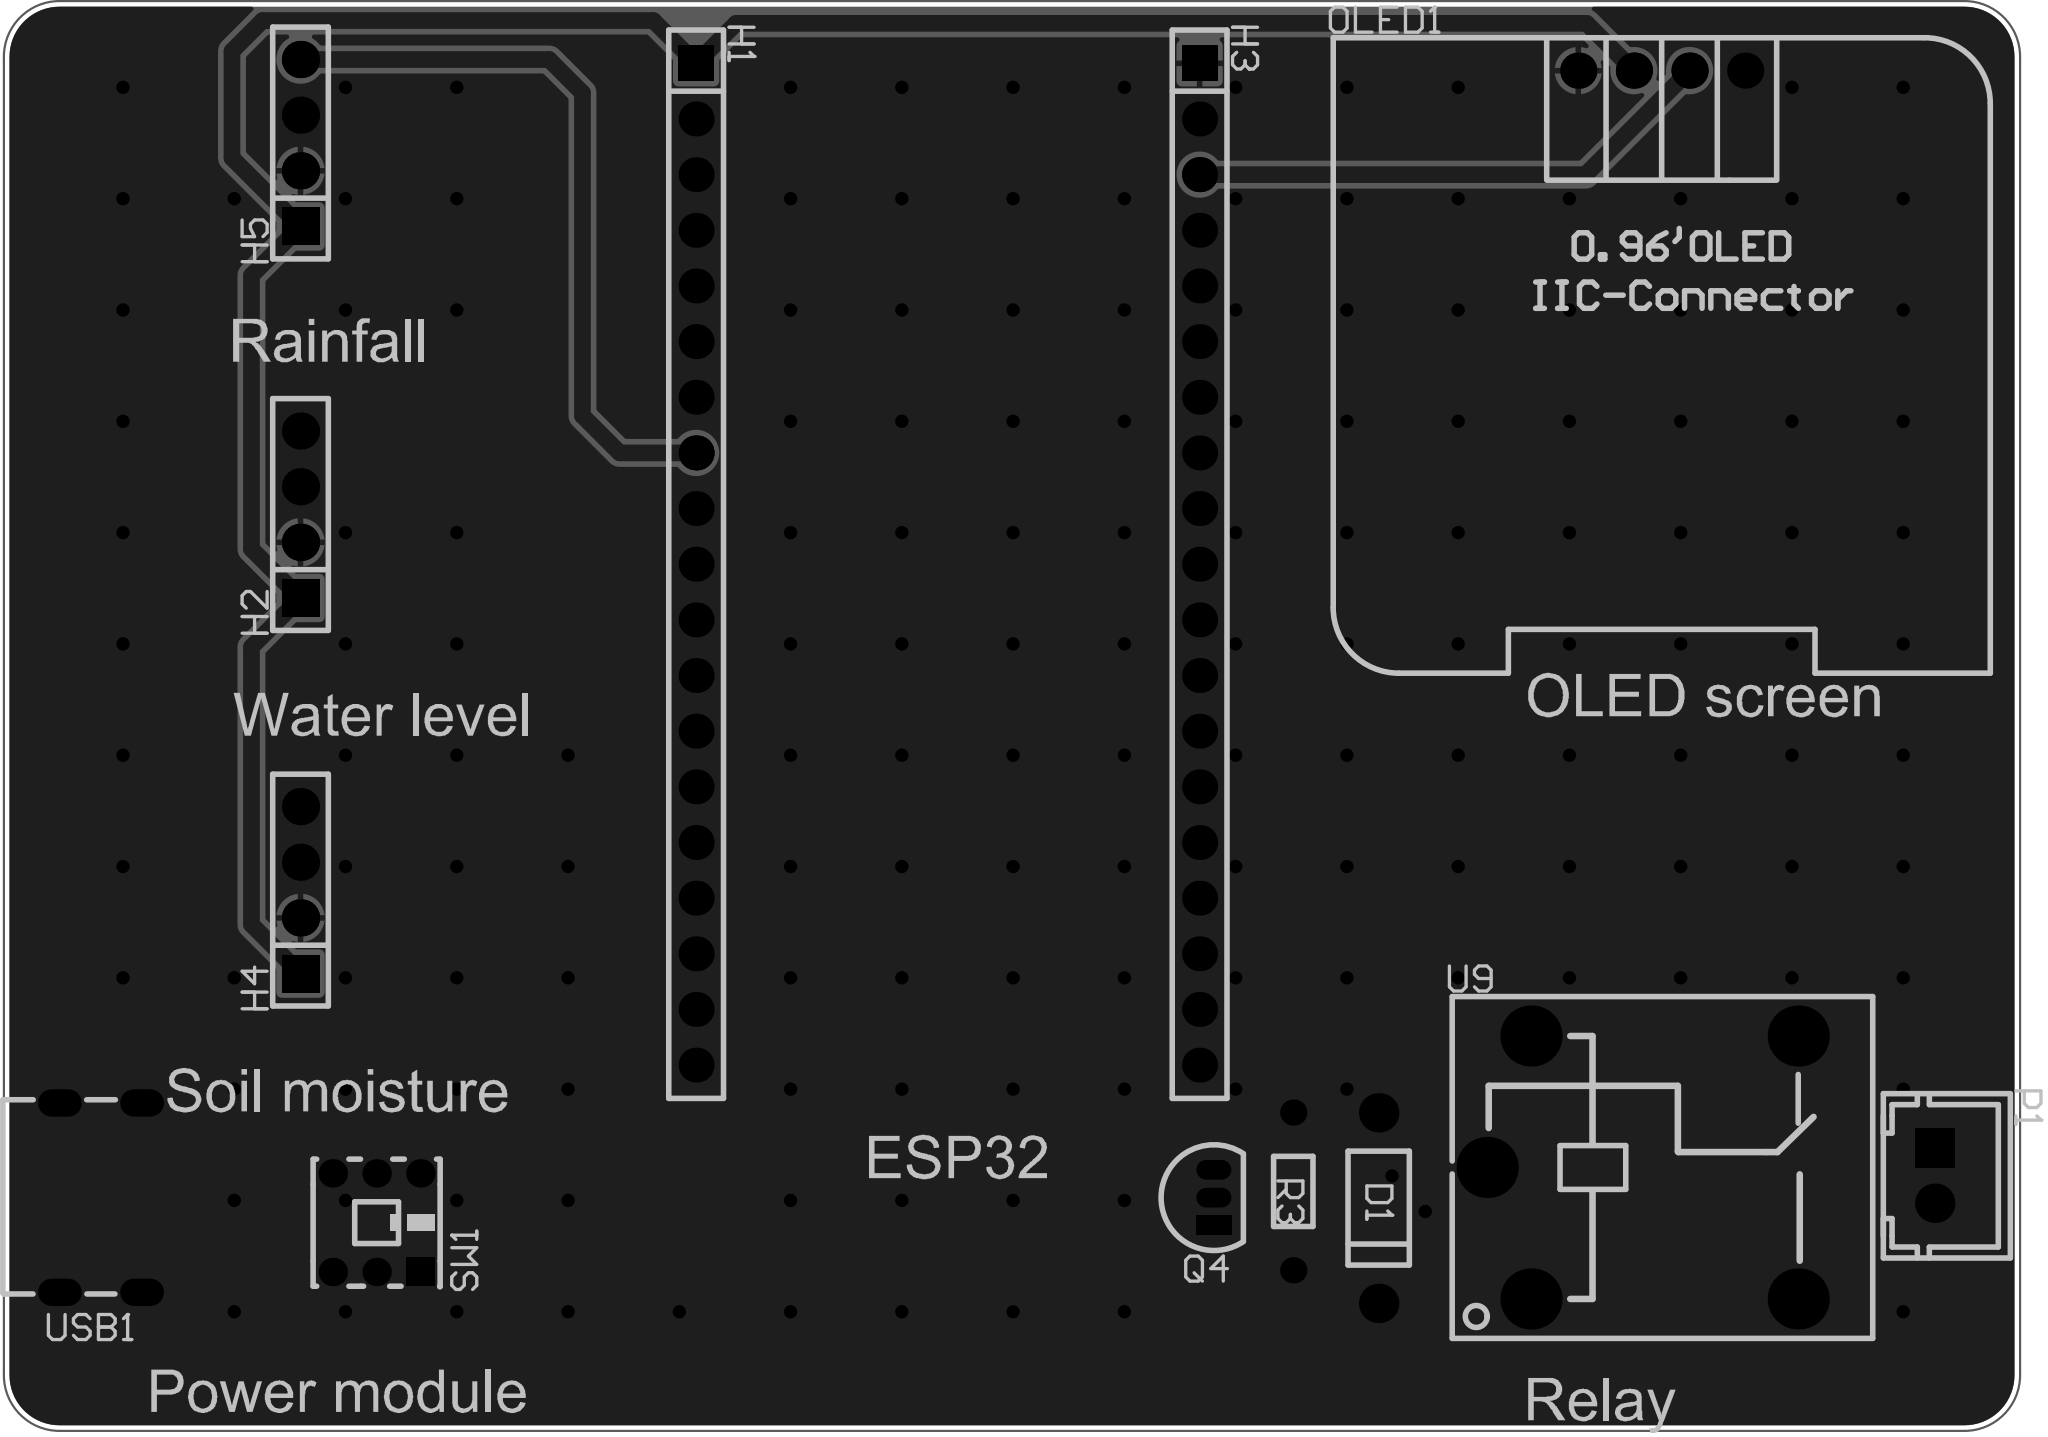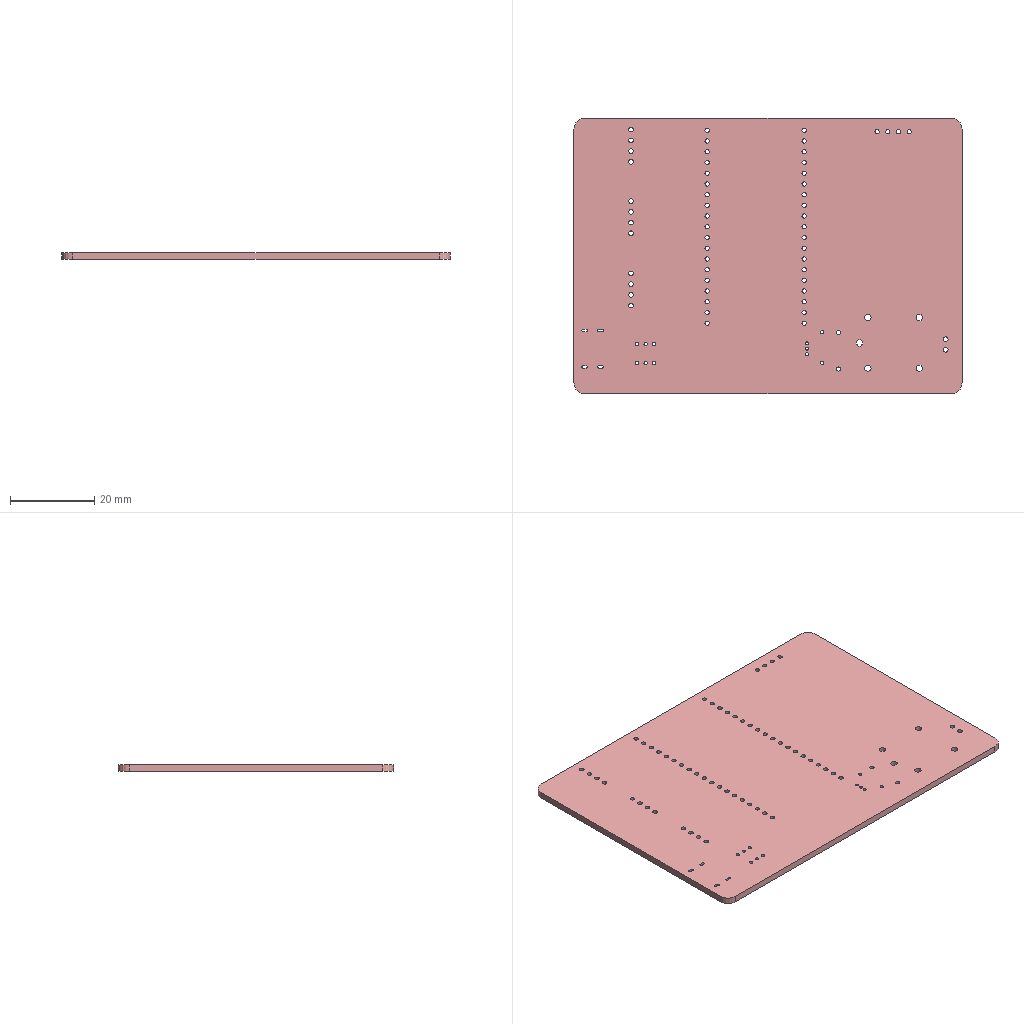Circuit board layout | Altium Designer | box 92.1 x 65.3 x 1.6 mm
Layer stack:
# Altium Designer layer stack of  (unit mm; dielectric type: 0 none, 1 core, 2 prepreg, 3 surface material)
index,name,kind,layer,copper_thickness_mm,dielectric_type,dielectric_thickness_mm,dielectric_material,dielectric_constant
0,Top Paste Mask Layer,other,,,,,,
1,Top Silkscreen Layer,other,,,,,,
2,Top Solder Mask Layer,dielectric,,,3,0.01,,3.3
3,Top Layer,copper,Top Layer,0.035,,,,
4,Dielectric1,dielectric,,,3,1.51,FR4,4.5
5,Bottom Layer,copper,Bottom Layer,0.035,,,,
6,Bottom Solder Mask Layer,dielectric,,,3,0.01,,3.3
7,Bottom Silkscreen Layer,other,,,,,,
8,Bottom Paste Mask Layer,other,,,,,,
# drill layer pairs: low layer,high layer
drill_pair,Top Layer,Bottom Layer
Part placement:
Designator,Comment,Layer,Footprint,Center-X(mm),Center-Y(mm),Rotation
U9,SRD-12VDC-SL-C,TopLayer,RELAY-TH_SRD-XXVDC-XL-C,159.914,102.087,0
P1,WAFER-XH254Z-2A,TopLayer,CONN-TH_2P-P2.50_XH-2A_3045048,173.249,101.706,270
SW1,5.8 WSPT,TopLayer,SW-TH_6P-L5.8-W5.8-P2.00-LS4.5-TL_K8-5851E-L1,102.108,99.568,180
D1,,TopLayer,DO_1N4007,147.859,100.233,90
Q4,,TopLayer,S8050_TO_92,140.335,100.711,90
R3,1K,TopLayer,Res_1/8W,143.959,100.995,270
H1,C2897382,TopLayer,HDR-TH_19P-P2.54-V-F,116.696,129.619,270
H3,C2897382,TopLayer,HDR-TH_19P-P2.54-V-F,139.683,129.619,270
OLED1,,TopLayer,0.96OLED_4P,160.782,152.146,0
USB1,,TopLayer,USB__TYPE-C-6P,89.789,100.711,270
H2,,TopLayer,HDR-TH_4P-P2.54-V-F,98.632,131.888,90
H4,,TopLayer,HDR-TH_4P-P2.54-V-F,98.632,114.747,90
H5,,TopLayer,HDR-TH_4P-P2.54-V-F,98.632,148.844,90
Pad and via stacks:
# Altium Designer via and pad stacks of  (unit mm). Each distinct definition once, with the count of objects using it.
# via: kind,start_layer,end_layer,hole_mm,diameter_mm,mode(0 simple;1 top-mid-bottom;2 full stack),diameter_per_layer,count,example_net
# pad: kind,layer,hole_mm,hole_type(0 round;1 square;2 slot),plating,top_size,top_shape(1 round;2 rect;3 octagon;9 rounded rect),mid_size,bottom_size,mode,footprint,size_per_layer,count,example
pad,Multi-Layer,1.524,0,plated,2.794x2.794,1,2.794x2.794,2.794x2.794,0,RELAY-TH_SRD-XXVDC-XL-C,,5,U9.2
pad,Multi-Layer,1.1,0,plated,1.8x1.8,1,1.8x1.8,1.8x1.8,0,CONN-TH_2P-P2.50_XH-2A_3045048,,1,P1.2
pad,Multi-Layer,1.1,0,plated,1.8x1.8,2,1.8x1.8,1.8x1.8,0,CONN-TH_2P-P2.50_XH-2A_3045048,,1,P1.1
pad,Multi-Layer,0.8,0,plated,1.3x1.3,2,1.3x1.3,1.3x1.3,0,SW-TH_6P-L5.8-W5.8-P2.00-LS4.5-TL_K8-5851E-L1,,1,SW1.1
pad,Multi-Layer,0.8,0,plated,1.3x1.3,1,1.3x1.3,1.3x1.3,0,SW-TH_6P-L5.8-W5.8-P2.00-LS4.5-TL_K8-5851E-L1,,5,SW1.2
pad,Multi-Layer,1,0,plated,1.8x1.8,1,1.8x1.8,1.8x1.8,0,DO_1N4007,,2,D1.1
pad,Multi-Layer,0.701,0,plated,0.8992x1.6,2,0.8992x1.6,0.8992x1.6,0,S8050_TO_92,,1,Q4.1
pad,Multi-Layer,0.701,0,plated,0.8992x1.6,1,0.8992x1.6,0.8992x1.6,0,S8050_TO_92,,2,Q4.2
pad,Multi-Layer,0.8001,0,plated,1.199x1.199,1,1.199x1.199,1.199x1.199,0,Res_1/8W,,2,R3.1
pad,Multi-Layer,1.05,0,plated,1.6x1.6,1,1.6x1.6,1.6x1.6,0,HDR-TH_19P-P2.54-V-F,,36,H1.19
pad,Multi-Layer,1.05,0,plated,1.6x1.6,2,1.6x1.6,1.6x1.6,0,HDR-TH_19P-P2.54-V-F,,2,H1.1
pad,Multi-Layer,1,0,plated,1.65x1.65,1,1.65x1.65,1.65x1.65,0,0.96OLED_4P,,4,OLED1.4
pad,Multi-Layer,0.6,2,plated,1.25x2,1,1.25x2,1.25x2,0,USB_ TYPE-C-6P,,4,USB1.8
pad,Multi-Layer,1.1,0,plated,1.7x1.7,2,1.7x1.7,1.7x1.7,0,HDR-TH_4P-P2.54-V-F,,3,H2.1
pad,Multi-Layer,1.1,0,plated,1.7x1.7,1,1.7x1.7,1.7x1.7,0,HDR-TH_4P-P2.54-V-F,,9,H2.2
pad,Top Layer,0,0,plated,0.7x1.2,2,0.7x1.2,0.7x1.2,0,USB_ TYPE-C-6P,,2,USB1.A5
pad,Top Layer,0,0,plated,0.8x1.2,2,0.8x1.2,0.8x1.2,0,USB_ TYPE-C-6P,,2,USB1.B9
pad,Top Layer,0,0,plated,0.9x1.2,2,0.9x1.2,0.9x1.2,0,USB_ TYPE-C-6P,,2,USB1.B12
via,Top Layer,Bottom Layer,0.3048,0.61,0,,158,GND
Copper pours:
name,layer,net,type(0 solid;1 hatched;2 none)
Top Layer-GND,Top Layer,GND,0
Bottom Layer-GND,Bottom Layer,GND,0